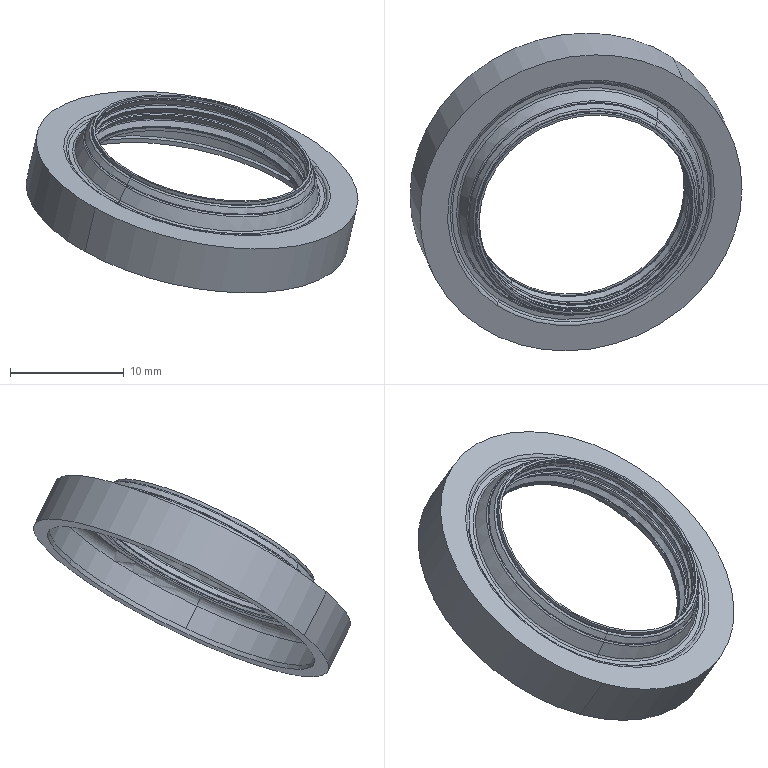Part | SolidWorks | features BaseBody 1 | 1 solid | 95 faces | box 29.233 x 27.963 x 17.759 mm | volume 697.835 mm3 | torus 45 | cone 24 | cylinder 16 | plane 10 | commonest cylinder face diameters 19.255 x4 19.055 x2 19.655 x2 22.5 x2 26.2 x2 27.2 x2